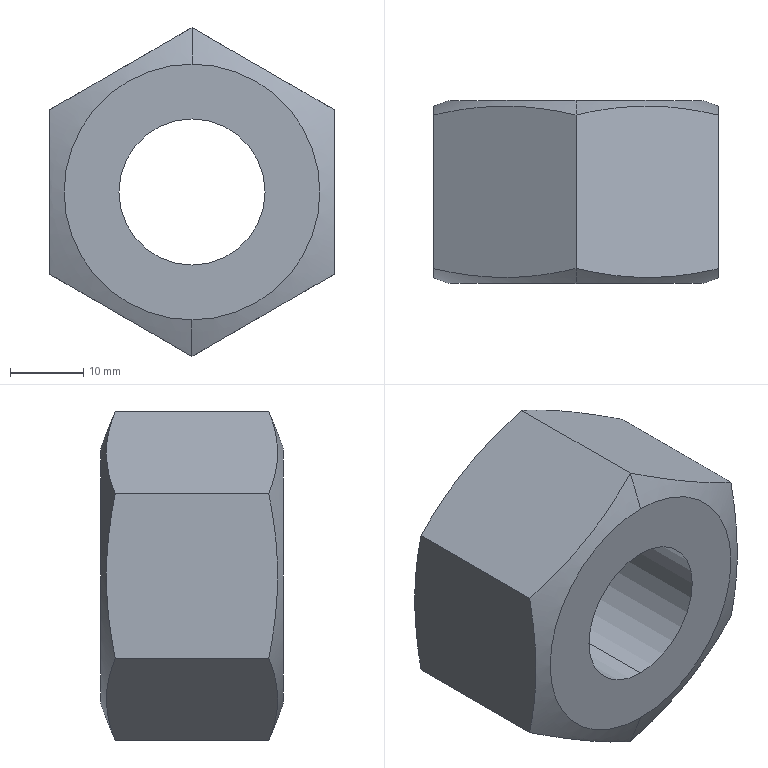Part | SolidWorks | features Extrusion 1, MirrorPattern 1, RevCut 1 | 1 solid | 14 faces | box 38.971 x 25 x 45 mm | volume 24565 mm3 | plane 8 | torus 4 | cylinder 2 | commonest cylinder face diameters 20 x2